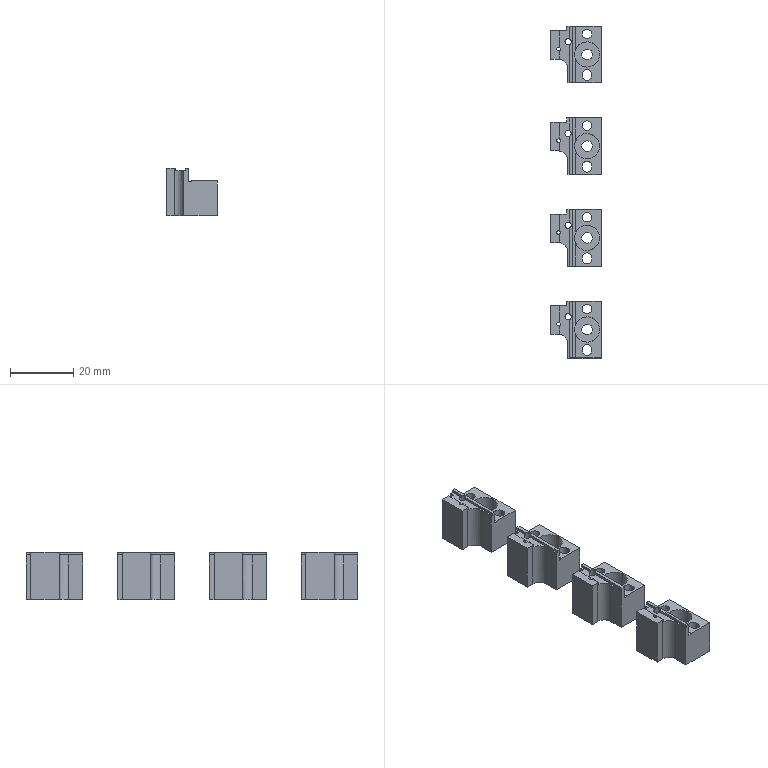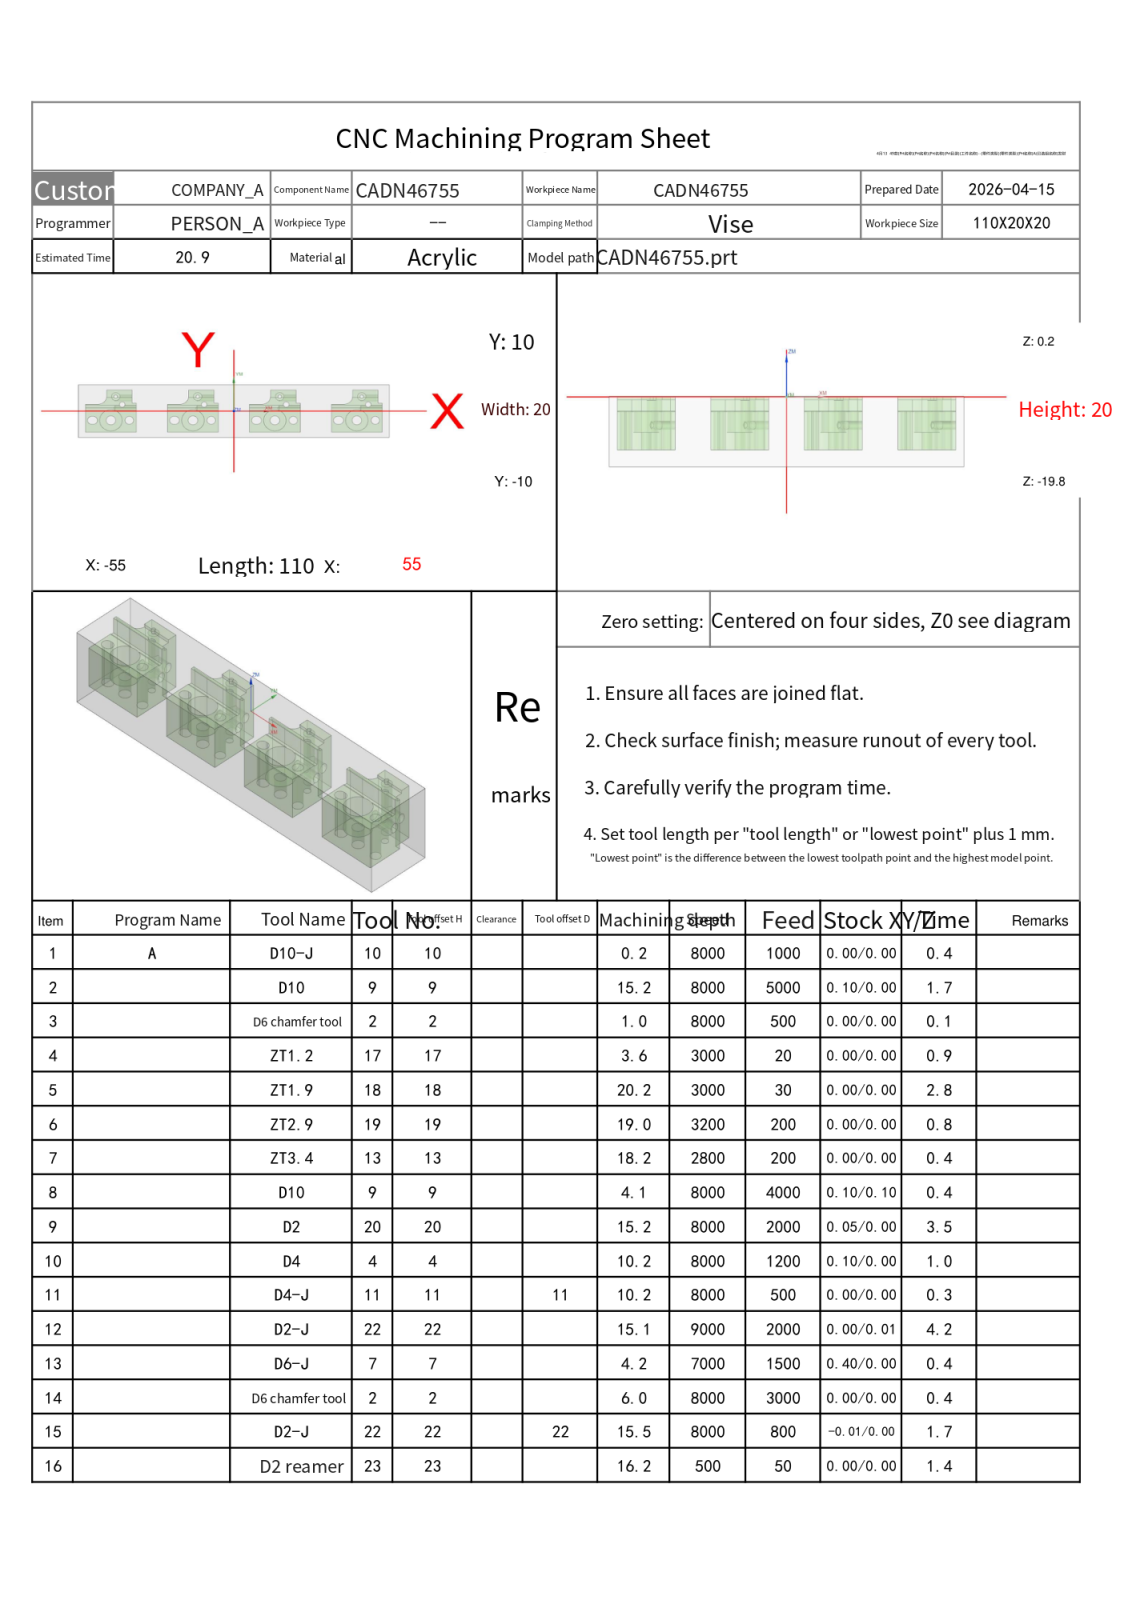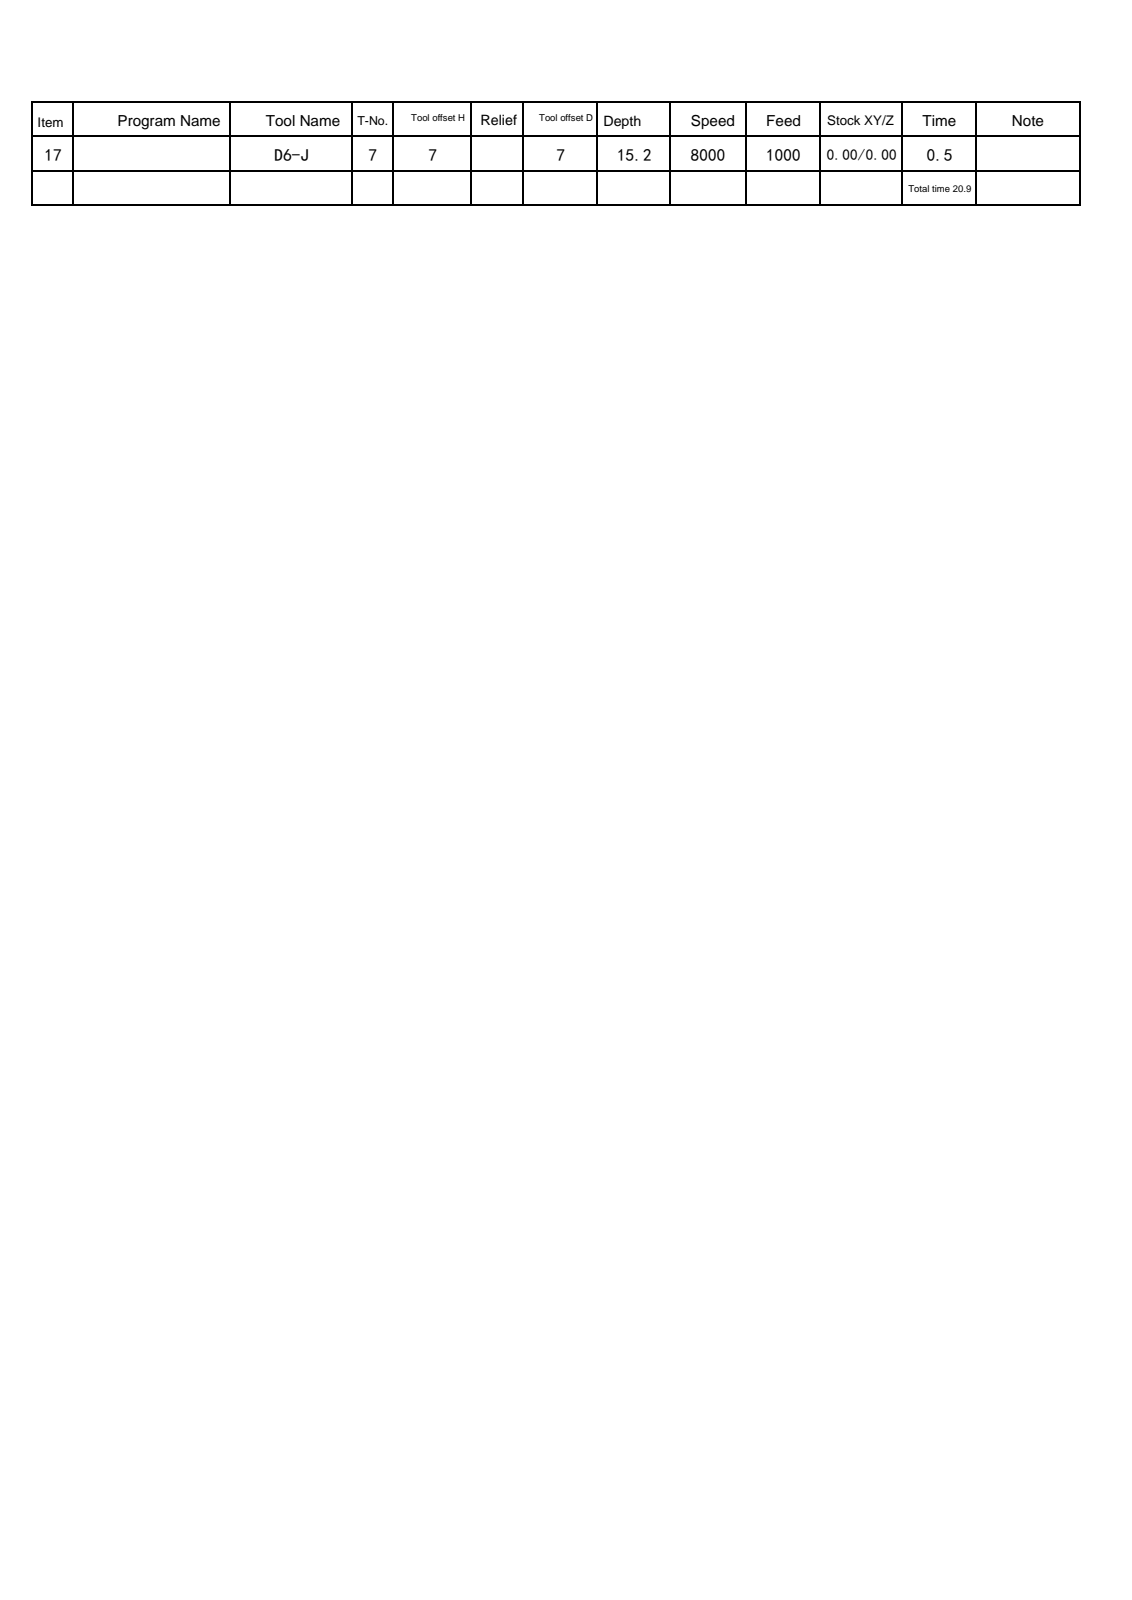NC program | NX | posted by the shop | part box 16 x 105 x 15 mm
Lines 1403 to 2192 of 25120:
N9 T20 M06
(D2  D=2. R=0. H=20 ce=0.10 di=0.00)
G00 G90 G54 X-50. Y-3.9 M03 S6000
G43 H20 Z20.
M08
Z-3.5
G01 X-49.75 Z-3.507 F600.
G03 X-49.35 Y-3.5 Z-3.525 I0.0 J.4
X-49.75 Y-3.1 Z-3.543 I-.4 J0.0
G01 X-50.25 Z-3.557
G03 X-50.65 Y-3.5 Z-3.574 I0.0 J-.4
X-50.559 Y-3.754 Z-3.582 I.4 J0.0
X-50.25 Y-3.9 Z-3.592 I.309 J.254
G01 X-49.75 Z-3.606
G03 X-49.35 Y-3.5 Z-3.624 I0.0 J.4
X-49.75 Y-3.1 Z-3.642 I-.4 J0.0
G01 X-50.25 Z-3.656
G03 X-50.65 Y-3.5 Z-3.673 I0.0 J-.4
X-50.559 Y-3.754 Z-3.681 I.4 J0.0
X-50.25 Y-3.9 Z-3.691 I.309 J.254
G01 X-49.75 Z-3.705
G03 X-49.35 Y-3.5 Z-3.723 I0.0 J.4
X-49.75 Y-3.1 Z-3.741 I-.4 J0.0
G01 X-50.25 Z-3.755
G03 X-50.65 Y-3.5 Z-3.773 I0.0 J-.4
X-50.559 Y-3.754 Z-3.78 I.4 J0.0
X-50.25 Y-3.9 Z-3.79 I.309 J.254
G01 X-49.75 Z-3.804
G03 X-49.35 Y-3.5 Z-3.822 I0.0 J.4
X-49.75 Y-3.1 Z-3.84 I-.4 J0.0
G01 X-50.25 Z-3.854
G03 X-50.65 Y-3.5 Z-3.872 I0.0 J-.4
X-50.559 Y-3.754 Z-3.88 I.4 J0.0
X-50.25 Y-3.9 Z-3.889 I.309 J.254
G01 X-49.75 Z-3.904
G03 X-49.35 Y-3.5 Z-3.921 I0.0 J.4
X-49.75 Y-3.1 Z-3.939 I-.4 J0.0
G01 X-50.25 Z-3.953
G03 X-50.65 Y-3.5 Z-3.971 I0.0 J-.4
X-50.559 Y-3.754 Z-3.979 I.4 J0.0
X-50.25 Y-3.9 Z-3.989 I.309 J.254
G01 X-49.75 Z-4.003
G03 X-49.35 Y-3.5 Z-4.02 I0.0 J.4
X-49.75 Y-3.1 Z-4.038 I-.4 J0.0
G01 X-50.25 Z-4.052
G03 X-50.65 Y-3.5 Z-4.07 I0.0 J-.4
X-50.559 Y-3.754 Z-4.078 I.4 J0.0
X-50.25 Y-3.9 Z-4.088 I.309 J.254
G01 X-49.75 Z-4.102
G03 X-49.35 Y-3.5 Z-4.12 I0.0 J.4
X-49.75 Y-3.1 Z-4.137 I-.4 J0.0
G01 X-50.25 Z-4.151
G03 X-50.65 Y-3.5 Z-4.169 I0.0 J-.4
X-50.559 Y-3.754 Z-4.177 I.4 J0.0
X-50.25 Y-3.9 Z-4.187 I.309 J.254
G01 X-49.75 Z-4.201
G03 X-49.35 Y-3.5 Z-4.219 I0.0 J.4
X-49.75 Y-3.1 Z-4.236 I-.4 J0.0
G01 X-50.25 Z-4.251
G03 X-50.65 Y-3.5 Z-4.268 I0.0 J-.4
X-50.559 Y-3.754 Z-4.276 I.4 J0.0
X-50.25 Y-3.9 Z-4.286 I.309 J.254
G01 X-49.75 Z-4.3
G03 X-49.35 Y-3.5 Z-4.318 I0.0 J.4
X-49.75 Y-3.1 Z-4.336 I-.4 J0.0
G01 X-50.25 Z-4.35
G03 X-50.65 Y-3.5 Z-4.367 I0.0 J-.4
X-50.559 Y-3.754 Z-4.375 I.4 J0.0
X-50.25 Y-3.9 Z-4.385 I.309 J.254
G01 X-49.75 Z-4.399
G03 X-49.35 Y-3.5 Z-4.417 I0.0 J.4
X-49.75 Y-3.1 Z-4.435 I-.4 J0.0
G01 X-50.25 Z-4.449
G03 X-50.65 Y-3.5 Z-4.467 I0.0 J-.4
X-50.559 Y-3.754 Z-4.474 I.4 J0.0
X-50.25 Y-3.9 Z-4.484 I.309 J.254
G01 X-49.75 Z-4.498
G03 X-49.35 Y-3.5 Z-4.516 I0.0 J.4
X-49.75 Y-3.1 Z-4.534 I-.4 J0.0
G01 X-50.25 Z-4.548
G03 X-50.65 Y-3.5 Z-4.566 I0.0 J-.4
X-50.559 Y-3.754 Z-4.574 I.4 J0.0
X-50.25 Y-3.9 Z-4.583 I.309 J.254
G01 X-49.75 Z-4.598
G03 X-49.35 Y-3.5 Z-4.615 I0.0 J.4
X-49.75 Y-3.1 Z-4.633 I-.4 J0.0
G01 X-50.25 Z-4.647
G03 X-50.65 Y-3.5 Z-4.665 I0.0 J-.4
X-50.559 Y-3.754 Z-4.673 I.4 J0.0
X-50.25 Y-3.9 Z-4.683 I.309 J.254
G01 X-49.75 Z-4.697
G03 X-49.35 Y-3.5 Z-4.714 I0.0 J.4
X-49.75 Y-3.1 Z-4.732 I-.4 J0.0
G01 X-50.25 Z-4.746
G03 X-50.65 Y-3.5 Z-4.764 I0.0 J-.4
X-50.559 Y-3.754 Z-4.772 I.4 J0.0
X-50.25 Y-3.9 Z-4.782 I.309 J.254
G01 X-49.75 Z-4.796
G03 X-49.35 Y-3.5 Z-4.814 I0.0 J.4
X-49.75 Y-3.1 Z-4.831 I-.4 J0.0
G01 X-50.25 Z-4.845
G03 X-50.65 Y-3.5 Z-4.863 I0.0 J-.4
X-50.559 Y-3.754 Z-4.871 I.4 J0.0
X-50.25 Y-3.9 Z-4.881 I.309 J.254
G01 X-49.75 Z-4.895
G03 X-49.35 Y-3.5 Z-4.913 I0.0 J.4
X-49.75 Y-3.1 Z-4.93 I-.4 J0.0
G01 X-50.25 Z-4.945
G03 X-50.65 Y-3.5 Z-4.962 I0.0 J-.4
X-50.559 Y-3.754 Z-4.97 I.4 J0.0
X-50.25 Y-3.9 Z-4.98 I.309 J.254
G01 X-49.75 Z-4.994
G03 X-49.35 Y-3.5 Z-5.012 I0.0 J.4
X-49.75 Y-3.1 Z-5.03 I-.4 J0.0
G01 X-50.25 Z-5.044
G03 X-50.65 Y-3.5 Z-5.061 I0.0 J-.4
X-50.559 Y-3.754 Z-5.069 I.4 J0.0
X-50.25 Y-3.9 Z-5.079 I.309 J.254
G01 X-49.75 Z-5.093
G03 X-49.35 Y-3.5 Z-5.111 I0.0 J.4
X-49.75 Y-3.1 Z-5.129 I-.4 J0.0
G01 X-50.25 Z-5.143
G03 X-50.65 Y-3.5 Z-5.161 I0.0 J-.4
X-50.559 Y-3.754 Z-5.168 I.4 J0.0
X-50.25 Y-3.9 Z-5.178 I.309 J.254
G01 X-49.75 Z-5.192
G03 X-49.35 Y-3.5 Z-5.21 I0.0 J.4
X-49.75 Y-3.1 Z-5.228 I-.4 J0.0
G01 X-50.25 Z-5.242
G03 X-50.65 Y-3.5 Z-5.26 I0.0 J-.4
X-50.559 Y-3.754 Z-5.267 I.4 J0.0
X-50.25 Y-3.9 Z-5.277 I.309 J.254
G01 X-49.75 Z-5.292
G03 X-49.35 Y-3.5 Z-5.309 I0.0 J.4
X-49.75 Y-3.1 Z-5.327 I-.4 J0.0
G01 X-50.25 Z-5.341
G03 X-50.65 Y-3.5 Z-5.359 I0.0 J-.4
X-50.559 Y-3.754 Z-5.367 I.4 J0.0
X-50.25 Y-3.9 Z-5.377 I.309 J.254
G01 X-49.75 Z-5.391
G03 X-49.35 Y-3.5 Z-5.408 I0.0 J.4
X-49.75 Y-3.1 Z-5.426 I-.4 J0.0
G01 X-50.25 Z-5.44
G03 X-50.65 Y-3.5 Z-5.458 I0.0 J-.4
X-50.559 Y-3.754 Z-5.466 I.4 J0.0
X-50.25 Y-3.9 Z-5.476 I.309 J.254
G01 X-49.75 Z-5.49
G03 X-49.35 Y-3.5 Z-5.508 I0.0 J.4
X-49.75 Y-3.1 Z-5.525 I-.4 J0.0
G01 X-50.25 Z-5.539
G03 X-50.65 Y-3.5 Z-5.557 I0.0 J-.4
X-50.559 Y-3.754 Z-5.565 I.4 J0.0
X-50.25 Y-3.9 Z-5.575 I.309 J.254
G01 X-49.75 Z-5.589
G03 X-49.35 Y-3.5 Z-5.607 I0.0 J.4
X-49.75 Y-3.1 Z-5.624 I-.4 J0.0
G01 X-50.25 Z-5.639
G03 X-50.65 Y-3.5 Z-5.656 I0.0 J-.4
X-50.559 Y-3.754 Z-5.664 I.4 J0.0
X-50.25 Y-3.9 Z-5.674 I.309 J.254
G01 X-49.75 Z-5.688
G03 X-49.35 Y-3.5 Z-5.706 I0.0 J.4
X-49.75 Y-3.1 Z-5.724 I-.4 J0.0
G01 X-50.25 Z-5.738
G03 X-50.65 Y-3.5 Z-5.755 I0.0 J-.4
X-50.559 Y-3.754 Z-5.763 I.4 J0.0
X-50.25 Y-3.9 Z-5.773 I.309 J.254
G01 X-49.75 Z-5.787
G03 X-49.35 Y-3.5 Z-5.805 I0.0 J.4
X-49.75 Y-3.1 Z-5.823 I-.4 J0.0
G01 X-50.25 Z-5.837
G03 X-50.65 Y-3.5 Z-5.855 I0.0 J-.4
X-50.559 Y-3.754 Z-5.862 I.4 J0.0
X-50.25 Y-3.9 Z-5.872 I.309 J.254
G01 X-49.75 Z-5.886
G03 X-49.35 Y-3.5 Z-5.904 I0.0 J.4
X-49.75 Y-3.1 Z-5.922 I-.4 J0.0
G01 X-50.25 Z-5.936
G03 X-50.65 Y-3.5 Z-5.954 I0.0 J-.4
X-50.559 Y-3.754 Z-5.961 I.4 J0.0
X-50.25 Y-3.9 Z-5.971 I.309 J.254
G01 X-49.75 Z-5.986
G03 X-49.35 Y-3.5 Z-6.003 I0.0 J.4
X-49.75 Y-3.1 Z-6.021 I-.4 J0.0
G01 X-50.25 Z-6.035
G03 X-50.65 Y-3.5 Z-6.053 I0.0 J-.4
X-50.559 Y-3.754 Z-6.061 I.4 J0.0
X-50.25 Y-3.9 Z-6.071 I.309 J.254
G01 X-49.75 Z-6.085
G03 X-49.35 Y-3.5 Z-6.102 I0.0 J.4
X-49.75 Y-3.1 Z-6.12 I-.4 J0.0
G01 X-50.25 Z-6.134
G03 X-50.65 Y-3.5 Z-6.152 I0.0 J-.4
X-50.559 Y-3.754 Z-6.16 I.4 J0.0
X-50.25 Y-3.9 Z-6.17 I.309 J.254
G01 X-49.75 Z-6.184
G03 X-49.35 Y-3.5 Z-6.202 I0.0 J.4
X-49.75 Y-3.1 Z-6.219 I-.4 J0.0
G01 X-50.25 Z-6.233
G03 X-50.65 Y-3.5 Z-6.251 I0.0 J-.4
X-50.559 Y-3.754 Z-6.259 I.4 J0.0
X-50.25 Y-3.9 Z-6.269 I.309 J.254
G01 X-49.75 Z-6.283
G03 X-49.35 Y-3.5 Z-6.301 I0.0 J.4
X-49.75 Y-3.1 Z-6.318 I-.4 J0.0
G01 X-50.25 Z-6.332
G03 X-50.65 Y-3.5 Z-6.35 I0.0 J-.4
X-50.559 Y-3.754 Z-6.358 I.4 J0.0
X-50.25 Y-3.9 Z-6.368 I.309 J.254
G01 X-49.75 Z-6.382
G03 X-49.35 Y-3.5 Z-6.4 I0.0 J.4
X-49.75 Y-3.1 Z-6.418 I-.4 J0.0
G01 X-50.25 Z-6.432
G03 X-50.65 Y-3.5 Z-6.449 I0.0 J-.4
X-50.559 Y-3.754 Z-6.457 I.4 J0.0
X-50.25 Y-3.9 Z-6.467 I.309 J.254
G01 X-49.75 Z-6.481
G03 X-49.35 Y-3.5 Z-6.499 I0.0 J.4
X-49.75 Y-3.1 Z-6.517 I-.4 J0.0
G01 X-50.25 Z-6.531
G03 X-50.65 Y-3.5 Z-6.548 I0.0 J-.4
X-50.559 Y-3.754 Z-6.556 I.4 J0.0
X-50.25 Y-3.9 Z-6.566 I.309 J.254
G01 X-49.75 Z-6.58
G03 X-49.35 Y-3.5 Z-6.598 I0.0 J.4
X-49.75 Y-3.1 Z-6.616 I-.4 J0.0
G01 X-50.25 Z-6.63
G03 X-50.65 Y-3.5 Z-6.648 I0.0 J-.4
X-50.559 Y-3.754 Z-6.655 I.4 J0.0
X-50.25 Y-3.9 Z-6.665 I.309 J.254
G01 X-49.75 Z-6.679
G03 X-49.35 Y-3.5 Z-6.697 I0.0 J.4
X-49.75 Y-3.1 Z-6.715 I-.4 J0.0
G01 X-50.25 Z-6.729
G03 X-50.65 Y-3.5 Z-6.747 I0.0 J-.4
X-50.559 Y-3.754 Z-6.755 I.4 J0.0
X-50.25 Y-3.9 Z-6.764 I.309 J.254
G01 X-49.75 Z-6.779
G03 X-49.35 Y-3.5 Z-6.796 I0.0 J.4
X-49.75 Y-3.1 Z-6.814 I-.4 J0.0
G01 X-50.25 Z-6.828
G03 X-50.65 Y-3.5 Z-6.846 I0.0 J-.4
X-50.559 Y-3.754 Z-6.854 I.4 J0.0
X-50.25 Y-3.9 Z-6.864 I.309 J.254
G01 X-49.75 Z-6.878
G03 X-49.35 Y-3.5 Z-6.895 I0.0 J.4
X-49.75 Y-3.1 Z-6.913 I-.4 J0.0
G01 X-50.25 Z-6.927
G03 X-50.65 Y-3.5 Z-6.945 I0.0 J-.4
X-50.559 Y-3.754 Z-6.953 I.4 J0.0
X-50.25 Y-3.9 Z-6.963 I.309 J.254
G01 X-49.75 Z-6.977
G03 X-49.35 Y-3.5 Z-6.995 I0.0 J.4
X-49.75 Y-3.1 Z-7.012 I-.4 J0.0
G01 X-50.25 Z-7.026
G03 X-50.65 Y-3.5 Z-7.044 I0.0 J-.4
X-50.559 Y-3.754 Z-7.052 I.4 J0.0
X-50.25 Y-3.9 Z-7.062 I.309 J.254
G01 X-49.75 Z-7.076
G03 X-49.35 Y-3.5 Z-7.094 I0.0 J.4
X-49.75 Y-3.1 Z-7.111 I-.4 J0.0
G01 X-50.25 Z-7.126
G03 X-50.65 Y-3.5 Z-7.143 I0.0 J-.4
X-50.559 Y-3.754 Z-7.151 I.4 J0.0
X-50.25 Y-3.9 Z-7.161 I.309 J.254
G01 X-49.75 Z-7.175
G03 X-49.35 Y-3.5 Z-7.193 I0.0 J.4
X-49.75 Y-3.1 Z-7.211 I-.4 J0.0
G01 X-50.25 Z-7.225
G03 X-50.65 Y-3.5 Z-7.242 I0.0 J-.4
X-50.559 Y-3.754 Z-7.25 I.4 J0.0
X-50.25 Y-3.9 Z-7.26 I.309 J.254
G01 X-49.75 Z-7.274
G03 X-49.35 Y-3.5 Z-7.292 I0.0 J.4
X-49.75 Y-3.1 Z-7.31 I-.4 J0.0
G01 X-50.25 Z-7.324
G03 X-50.65 Y-3.5 Z-7.342 I0.0 J-.4
X-50.559 Y-3.754 Z-7.349 I.4 J0.0
X-50.25 Y-3.9 Z-7.359 I.309 J.254
G01 X-49.75 Z-7.373
G03 X-49.35 Y-3.5 Z-7.391 I0.0 J.4
X-49.75 Y-3.1 Z-7.409 I-.4 J0.0
G01 X-50.25 Z-7.423
G03 X-50.65 Y-3.5 Z-7.441 I0.0 J-.4
X-50.559 Y-3.754 Z-7.449 I.4 J0.0
X-50.25 Y-3.9 Z-7.458 I.309 J.254
G01 X-49.75 Z-7.473
G03 X-49.35 Y-3.5 Z-7.49 I0.0 J.4
X-49.75 Y-3.1 Z-7.508 I-.4 J0.0
G01 X-50.25 Z-7.522
G03 X-50.65 Y-3.5 Z-7.54 I0.0 J-.4
X-50.559 Y-3.754 Z-7.548 I.4 J0.0
X-50.25 Y-3.9 Z-7.558 I.309 J.254
G01 X-49.75 Z-7.572
G03 X-49.35 Y-3.5 Z-7.589 I0.0 J.4
X-49.75 Y-3.1 Z-7.607 I-.4 J0.0
G01 X-50.25 Z-7.621
G03 X-50.65 Y-3.5 Z-7.639 I0.0 J-.4
X-50.559 Y-3.754 Z-7.647 I.4 J0.0
X-50.25 Y-3.9 Z-7.657 I.309 J.254
G01 X-49.75 Z-7.671
G03 X-49.35 Y-3.5 Z-7.689 I0.0 J.4
X-49.75 Y-3.1 Z-7.706 I-.4 J0.0
G01 X-50.25 Z-7.72
G03 X-50.65 Y-3.5 Z-7.738 I0.0 J-.4
X-50.559 Y-3.754 Z-7.746 I.4 J0.0
X-50.25 Y-3.9 Z-7.756 I.309 J.254
G01 X-49.75 Z-7.77
G03 X-49.35 Y-3.5 Z-7.788 I0.0 J.4
X-49.75 Y-3.1 Z-7.805 I-.4 J0.0
G01 X-50.25 Z-7.82
G03 X-50.65 Y-3.5 Z-7.837 I0.0 J-.4
X-50.559 Y-3.754 Z-7.845 I.4 J0.0
X-50.25 Y-3.9 Z-7.855 I.309 J.254
G01 X-49.75 Z-7.869
G03 X-49.35 Y-3.5 Z-7.887 I0.0 J.4
X-49.75 Y-3.1 Z-7.905 I-.4 J0.0
G01 X-50.25 Z-7.919
G03 X-50.65 Y-3.5 Z-7.936 I0.0 J-.4
X-50.559 Y-3.754 Z-7.944 I.4 J0.0
X-50.25 Y-3.9 Z-7.954 I.309 J.254
G01 X-49.75 Z-7.968
G03 X-49.35 Y-3.5 Z-7.986 I0.0 J.4
X-49.75 Y-3.1 Z-8.004 I-.4 J0.0
G01 X-50.25 Z-8.018
G03 X-50.65 Y-3.5 Z-8.036 I0.0 J-.4
X-50.559 Y-3.754 Z-8.043 I.4 J0.0
X-50.25 Y-3.9 Z-8.053 I.309 J.254
G01 X-49.75 Z-8.067
G03 X-49.35 Y-3.5 Z-8.085 I0.0 J.4
X-49.75 Y-3.1 Z-8.103 I-.4 J0.0
G01 X-50.25 Z-8.117
G03 X-50.65 Y-3.5 Z-8.135 I0.0 J-.4
X-50.559 Y-3.754 Z-8.142 I.4 J0.0
X-50.25 Y-3.9 Z-8.152 I.309 J.254
G01 X-49.75 Z-8.167
G03 X-49.35 Y-3.5 Z-8.184 I0.0 J.4
X-49.75 Y-3.1 Z-8.202 I-.4 J0.0
G01 X-50.25 Z-8.216
G03 X-50.65 Y-3.5 Z-8.234 I0.0 J-.4
X-50.559 Y-3.754 Z-8.242 I.4 J0.0
X-50.25 Y-3.9 Z-8.252 I.309 J.254
G01 X-49.75 Z-8.266
G03 X-49.35 Y-3.5 Z-8.283 I0.0 J.4
X-49.75 Y-3.1 Z-8.301 I-.4 J0.0
G01 X-50.25 Z-8.315
G03 X-50.65 Y-3.5 Z-8.333 I0.0 J-.4
X-50.559 Y-3.754 Z-8.341 I.4 J0.0
X-50.25 Y-3.9 Z-8.351 I.309 J.254
G01 X-49.75 Z-8.365
G03 X-49.35 Y-3.5 Z-8.383 I0.0 J.4
X-49.75 Y-3.1 Z-8.4 I-.4 J0.0
G01 X-50.25 Z-8.414
G03 X-50.65 Y-3.5 Z-8.432 I0.0 J-.4
X-50.559 Y-3.754 Z-8.44 I.4 J0.0
X-50.25 Y-3.9 Z-8.45 I.309 J.254
G01 X-49.75 Z-8.464
G03 X-49.35 Y-3.5 Z-8.482 I0.0 J.4
X-49.75 Y-3.1 Z-8.499 I-.4 J0.0
G01 X-50.25 Z-8.514
G03 X-50.65 Y-3.5 Z-8.531 I0.0 J-.4
X-50.559 Y-3.754 Z-8.539 I.4 J0.0
X-50.25 Y-3.9 Z-8.549 I.309 J.254
G01 X-49.75 Z-8.563
G03 X-49.35 Y-3.5 Z-8.581 I0.0 J.4
X-49.75 Y-3.1 Z-8.599 I-.4 J0.0
G01 X-50.25 Z-8.613
G03 X-50.65 Y-3.5 Z-8.63 I0.0 J-.4
X-50.559 Y-3.754 Z-8.638 I.4 J0.0
X-50.25 Y-3.9 Z-8.648 I.309 J.254
G01 X-49.75 Z-8.662
G03 X-49.35 Y-3.5 Z-8.68 I0.0 J.4
X-49.75 Y-3.1 Z-8.698 I-.4 J0.0
G01 X-50.25 Z-8.712
G03 X-50.65 Y-3.5 Z-8.73 I0.0 J-.4
X-50.559 Y-3.754 Z-8.737 I.4 J0.0
X-50.25 Y-3.9 Z-8.747 I.309 J.254
G01 X-49.75 Z-8.761
G03 X-49.35 Y-3.5 Z-8.779 I0.0 J.4
X-49.75 Y-3.1 Z-8.797 I-.4 J0.0
G01 X-50.25 Z-8.811
G03 X-50.65 Y-3.5 Z-8.829 I0.0 J-.4
X-50.559 Y-3.754 Z-8.836 I.4 J0.0
X-50.25 Y-3.9 Z-8.846 I.309 J.254
G01 X-49.75 Z-8.861
G03 X-49.35 Y-3.5 Z-8.878 I0.0 J.4
X-49.75 Y-3.1 Z-8.896 I-.4 J0.0
G01 X-50.25 Z-8.91
G03 X-50.65 Y-3.5 Z-8.928 I0.0 J-.4
X-50.559 Y-3.754 Z-8.936 I.4 J0.0
X-50.25 Y-3.9 Z-8.946 I.309 J.254
G01 X-49.75 Z-8.96
G03 X-49.35 Y-3.5 Z-8.977 I0.0 J.4
X-49.75 Y-3.1 Z-8.995 I-.4 J0.0
G01 X-50.25 Z-9.009
G03 X-50.65 Y-3.5 Z-9.027 I0.0 J-.4
X-50.559 Y-3.754 Z-9.035 I.4 J0.0
X-50.25 Y-3.9 Z-9.045 I.309 J.254
G01 X-49.75 Z-9.059
G03 X-49.35 Y-3.5 Z-9.077 I0.0 J.4
X-49.75 Y-3.1 Z-9.094 I-.4 J0.0
G01 X-50.25 Z-9.108
G03 X-50.65 Y-3.5 Z-9.126 I0.0 J-.4
X-50.559 Y-3.754 Z-9.134 I.4 J0.0
X-50.25 Y-3.9 Z-9.144 I.309 J.254
G01 X-49.75 Z-9.158
G03 X-49.35 Y-3.5 Z-9.176 I0.0 J.4
X-49.75 Y-3.1 Z-9.193 I-.4 J0.0
G01 X-50.25 Z-9.207
G03 X-50.65 Y-3.5 Z-9.225 I0.0 J-.4
X-50.559 Y-3.754 Z-9.233 I.4 J0.0
X-50.25 Y-3.9 Z-9.243 I.309 J.254
G01 X-49.75 Z-9.257
G03 X-49.35 Y-3.5 Z-9.275 I0.0 J.4
X-49.75 Y-3.1 Z-9.293 I-.4 J0.0
G01 X-50.25 Z-9.307
G03 X-50.65 Y-3.5 Z-9.324 I0.0 J-.4
X-50.559 Y-3.754 Z-9.332 I.4 J0.0
X-50.25 Y-3.9 Z-9.342 I.309 J.254
G01 X-49.75 Z-9.356
G03 X-49.35 Y-3.5 Z-9.374 I0.0 J.4
X-49.75 Y-3.1 Z-9.392 I-.4 J0.0
G01 X-50.25 Z-9.406
G03 X-50.65 Y-3.5 Z-9.423 I0.0 J-.4
X-50.559 Y-3.754 Z-9.431 I.4 J0.0
X-50.25 Y-3.9 Z-9.441 I.309 J.254
G01 X-49.75 Z-9.455
G03 X-49.35 Y-3.5 Z-9.473 I0.0 J.4
X-49.75 Y-3.1 Z-9.491 I-.4 J0.0
G01 X-50.25 Z-9.505
G03 X-50.65 Y-3.5 Z-9.523 I0.0 J-.4
X-50.559 Y-3.754 Z-9.53 I.4 J0.0
X-50.25 Y-3.9 Z-9.54 I.309 J.254
G01 X-49.75 Z-9.554
G03 X-49.35 Y-3.5 Z-9.572 I0.0 J.4
X-49.75 Y-3.1 Z-9.59 I-.4 J0.0
G01 X-50.25 Z-9.604
G03 X-50.65 Y-3.5 Z-9.622 I0.0 J-.4
X-50.559 Y-3.754 Z-9.63 I.4 J0.0
X-50.25 Y-3.9 Z-9.639 I.309 J.254
G01 X-49.75 Z-9.654
G03 X-49.35 Y-3.5 Z-9.671 I0.0 J.4
X-49.75 Y-3.1 Z-9.689 I-.4 J0.0
G01 X-50.25 Z-9.703
G03 X-50.65 Y-3.5 Z-9.721 I0.0 J-.4
X-50.559 Y-3.754 Z-9.729 I.4 J0.0
X-50.25 Y-3.9 Z-9.739 I.309 J.254
G01 X-49.75 Z-9.753
G03 X-49.35 Y-3.5 Z-9.77 I0.0 J.4
X-49.75 Y-3.1 Z-9.788 I-.4 J0.0
G01 X-50.25 Z-9.802
G03 X-50.65 Y-3.5 Z-9.82 I0.0 J-.4
X-50.559 Y-3.754 Z-9.828 I.4 J0.0
X-50.25 Y-3.9 Z-9.838 I.309 J.254
G01 X-49.75 Z-9.852
G03 X-49.35 Y-3.5 Z-9.87 I0.0 J.4
X-49.75 Y-3.1 Z-9.887 I-.4 J0.0
G01 X-50.25 Z-9.901
G03 X-50.65 Y-3.5 Z-9.919 I0.0 J-.4
X-50.559 Y-3.754 Z-9.927 I.4 J0.0
X-50.25 Y-3.9 Z-9.937 I.309 J.254
G01 X-49.75 Z-9.951
G03 X-49.35 Y-3.5 Z-9.969 I0.0 J.4
X-49.75 Y-3.1 Z-9.986 I-.4 J0.0
G01 X-50.25 Z-10.001
G03 X-50.65 Y-3.5 Z-10.018 I0.0 J-.4
X-50.559 Y-3.754 Z-10.026 I.4 J0.0
X-50.25 Y-3.9 Z-10.036 I.309 J.254
G01 X-49.75 Z-10.05
G03 X-49.35 Y-3.5 Z-10.068 I0.0 J.4
X-49.75 Y-3.1 Z-10.086 I-.4 J0.0
G01 X-50.25 Z-10.1
G03 X-50.65 Y-3.5 Z-10.117 I0.0 J-.4
X-50.559 Y-3.754 Z-10.125 I.4 J0.0
X-50.25 Y-3.9 Z-10.135 I.309 J.254
G01 X-49.75 Z-10.149
G03 X-49.35 Y-3.5 Z-10.167 I0.0 J.4
X-49.75 Y-3.1 Z-10.185 I-.4 J0.0
G01 X-50.25 Z-10.199
G03 X-50.65 Y-3.5 Z-10.217 I0.0 J-.4
X-50.559 Y-3.754 Z-10.224 I.4 J0.0
X-50.25 Y-3.9 Z-10.234 I.309 J.254
G01 X-49.75 Z-10.248
G03 X-49.35 Y-3.5 Z-10.266 I0.0 J.4
X-49.75 Y-3.1 Z-10.284 I-.4 J0.0
G01 X-50.25 Z-10.298
G03 X-50.65 Y-3.5 Z-10.316 I0.0 J-.4
X-50.559 Y-3.754 Z-10.324 I.4 J0.0
X-50.25 Y-3.9 Z-10.333 I.309 J.254
G01 X-49.75 Z-10.348
G03 X-49.35 Y-3.5 Z-10.365 I0.0 J.4
X-49.75 Y-3.1 Z-10.383 I-.4 J0.0
G01 X-50.25 Z-10.397
G03 X-50.65 Y-3.5 Z-10.415 I0.0 J-.4
X-50.559 Y-3.754 Z-10.423 I.4 J0.0
X-50.25 Y-3.9 Z-10.433 I.309 J.254
G01 X-49.75 Z-10.447
G03 X-49.35 Y-3.5 Z-10.464 I0.0 J.4
X-49.75 Y-3.1 Z-10.482 I-.4 J0.0
G01 X-50.25 Z-10.496
G03 X-50.65 Y-3.5 Z-10.514 I0.0 J-.4
X-50.559 Y-3.754 Z-10.522 I.4 J0.0
X-50.25 Y-3.9 Z-10.532 I.309 J.254
G01 X-49.75 Z-10.546
G03 X-49.35 Y-3.5 Z-10.564 I0.0 J.4
X-49.75 Y-3.1 Z-10.581 I-.4 J0.0
G01 X-50.25 Z-10.595
G03 X-50.65 Y-3.5 Z-10.613 I0.0 J-.4
X-50.559 Y-3.754 Z-10.621 I.4 J0.0
X-50.25 Y-3.9 Z-10.631 I.309 J.254
G01 X-49.75 Z-10.645
G03 X-49.35 Y-3.5 Z-10.663 I0.0 J.4
X-49.75 Y-3.1 Z-10.68 I-.4 J0.0
G01 X-50.25 Z-10.695
G03 X-50.65 Y-3.5 Z-10.712 I0.0 J-.4
X-50.559 Y-3.754 Z-10.72 I.4 J0.0
X-50.25 Y-3.9 Z-10.73 I.309 J.254
G01 X-49.75 Z-10.744
G03 X-49.35 Y-3.5 Z-10.762 I0.0 J.4
X-49.75 Y-3.1 Z-10.78 I-.4 J0.0
G01 X-50.25 Z-10.794
G03 X-50.65 Y-3.5 Z-10.811 I0.0 J-.4
X-50.559 Y-3.754 Z-10.819 I.4 J0.0
X-50.25 Y-3.9 Z-10.829 I.309 J.254
G01 X-49.75 Z-10.843
G03 X-49.35 Y-3.5 Z-10.861 I0.0 J.4
X-49.75 Y-3.1 Z-10.879 I-.4 J0.0
G01 X-50.25 Z-10.893
G03 X-50.65 Y-3.5 Z-10.911 I0.0 J-.4
X-50.559 Y-3.754 Z-10.918 I.4 J0.0
X-50.25 Y-3.9 Z-10.928 I.309 J.254
G01 X-49.75 Z-10.942
G03 X-49.35 Y-3.5 Z-10.96 I0.0 J.4
X-49.75 Y-3.1 Z-10.978 I-.4 J0.0
G01 X-50.25 Z-10.992
G03 X-50.65 Y-3.5 Z-11.01 I0.0 J-.4
X-50.559 Y-3.754 Z-11.017 I.4 J0.0
X-50.25 Y-3.9 Z-11.027 I.309 J.254
G01 X-49.75 Z-11.042
G03 X-49.35 Y-3.5 Z-11.059 I0.0 J.4
X-49.75 Y-3.1 Z-11.077 I-.4 J0.0
G01 X-50.25 Z-11.091
G03 X-50.65 Y-3.5 Z-11.109 I0.0 J-.4
X-50.559 Y-3.754 Z-11.117 I.4 J0.0
X-50.25 Y-3.9 Z-11.127 I.309 J.254
G01 X-49.75 Z-11.141
G03 X-49.35 Y-3.5 Z-11.158 I0.0 J.4
X-49.75 Y-3.1 Z-11.176 I-.4 J0.0
G01 X-50.25 Z-11.19
G03 X-50.65 Y-3.5 Z-11.208 I0.0 J-.4
X-50.559 Y-3.754 Z-11.216 I.4 J0.0
X-50.25 Y-3.9 Z-11.226 I.309 J.254
G01 X-49.75 Z-11.24
G03 X-49.35 Y-3.5 Z-11.258 I0.0 J.4
X-49.75 Y-3.1 Z-11.275 I-.4 J0.0
G01 X-50.25 Z-11.289
G03 X-50.65 Y-3.5 Z-11.307 I0.0 J-.4
X-50.559 Y-3.754 Z-11.315 I.4 J0.0
X-50.25 Y-3.9 Z-11.325 I.309 J.254
G01 X-49.75 Z-11.339
G03 X-49.35 Y-3.5 Z-11.357 I0.0 J.4
X-49.75 Y-3.1 Z-11.374 I-.4 J0.0
G01 X-50.25 Z-11.389
G03 X-50.65 Y-3.5 Z-11.406 I0.0 J-.4
X-50.559 Y-3.754 Z-11.414 I.4 J0.0
X-50.25 Y-3.9 Z-11.424 I.309 J.254
G01 X-49.75 Z-11.438
G03 X-49.35 Y-3.5 Z-11.456 I0.0 J.4
X-49.75 Y-3.1 Z-11.474 I-.4 J0.0
G01 X-50.25 Z-11.488
G03 X-50.65 Y-3.5 Z-11.505 I0.0 J-.4
X-50.559 Y-3.754 Z-11.513 I.4 J0.0
X-50.25 Y-3.9 Z-11.523 I.309 J.254
G01 X-49.75 Z-11.537
G03 X-49.35 Y-3.5 Z-11.555 I0.0 J.4
X-49.75 Y-3.1 Z-11.573 I-.4 J0.0
G01 X-50.25 Z-11.587
G03 X-50.65 Y-3.5 Z-11.605 I0.0 J-.4
X-50.559 Y-3.754 Z-11.612 I.4 J0.0
X-50.25 Y-3.9 Z-11.622 I.309 J.254
G01 X-49.75 Z-11.636
G03 X-49.35 Y-3.5 Z-11.654 I0.0 J.4
X-49.75 Y-3.1 Z-11.672 I-.4 J0.0
G01 X-50.25 Z-11.686
G03 X-50.65 Y-3.5 Z-11.704 I0.0 J-.4
X-50.559 Y-3.754 Z-11.711 I.4 J0.0
X-50.25 Y-3.9 Z-11.721 I.309 J.254
G01 X-49.75 Z-11.736
G03 X-49.35 Y-3.5 Z-11.753 I0.0 J.4
X-49.75 Y-3.1 Z-11.771 I-.4 J0.0
G01 X-50.25 Z-11.785
G03 X-50.65 Y-3.5 Z-11.803 I0.0 J-.4
X-50.559 Y-3.754 Z-11.811 I.4 J0.0
X-50.25 Y-3.9 Z-11.821 I.309 J.254
G01 X-49.75 Z-11.835
G03 X-49.35 Y-3.5 Z-11.852 I0.0 J.4
X-49.75 Y-3.1 Z-11.87 I-.4 J0.0
G01 X-50.25 Z-11.884
G03 X-50.65 Y-3.5 Z-11.902 I0.0 J-.4
X-50.559 Y-3.754 Z-11.91 I.4 J0.0
X-50.25 Y-3.9 Z-11.92 I.309 J.254
G01 X-49.75 Z-11.934
G03 X-49.35 Y-3.5 Z-11.952 I0.0 J.4
X-49.75 Y-3.1 Z-11.969 I-.4 J0.0
G01 X-50.25 Z-11.983
G03 X-50.65 Y-3.5 Z-12.001 I0.0 J-.4
X-50.559 Y-3.754 Z-12.009 I.4 J0.0
X-50.25 Y-3.9 Z-12.019 I.309 J.254
G01 X-49.75 Z-12.033
G03 X-49.35 Y-3.5 Z-12.051 I0.0 J.4
X-49.75 Y-3.1 Z-12.068 I-.4 J0.0
G01 X-50.25 Z-12.082
G03 X-50.65 Y-3.5 Z-12.1 I0.0 J-.4
X-50.559 Y-3.754 Z-12.108 I.4 J0.0
X-50.25 Y-3.9 Z-12.118 I.309 J.254
G01 X-49.75 Z-12.132
G03 X-49.35 Y-3.5 Z-12.15 I0.0 J.4
X-49.75 Y-3.1 Z-12.168 I-.4 J0.0
G01 X-50.25 Z-12.182
G03 X-50.65 Y-3.5 Z-12.199 I0.0 J-.4
X-50.559 Y-3.754 Z-12.207 I.4 J0.0
X-50.25 Y-3.9 Z-12.217 I.309 J.254
G01 X-49.75 Z-12.231
G03 X-49.35 Y-3.5 Z-12.249 I0.0 J.4
X-49.75 Y-3.1 Z-12.267 I-.4 J0.0
G01 X-50.25 Z-12.281
G03 X-50.65 Y-3.5 Z-12.298 I0.0 J-.4
X-50.559 Y-3.754 Z-12.306 I.4 J0.0
X-50.25 Y-3.9 Z-12.316 I.309 J.254
G01 X-49.75 Z-12.33
G03 X-49.35 Y-3.5 Z-12.348 I0.0 J.4
X-49.75 Y-3.1 Z-12.366 I-.4 J0.0
G01 X-50.25 Z-12.38
G03 X-50.65 Y-3.5 Z-12.398 I0.0 J-.4
X-50.559 Y-3.754 Z-12.405 I.4 J0.0
X-50.25 Y-3.9 Z-12.415 I.309 J.254
G01 X-49.75 Z-12.429
G03 X-49.35 Y-3.5 Z-12.447 I0.0 J.4
X-49.75 Y-3.1 Z-12.465 I-.4 J0.0
G01 X-50.25 Z-12.479
G03 X-50.65 Y-3.5 Z-12.497 I0.0 J-.4
X-50.559 Y-3.754 Z-12.505 I.4 J0.0
X-50.25 Y-3.9 Z-12.514 I.309 J.254
G01 X-49.75 Z-12.529
G03 X-49.35 Y-3.5 Z-12.546 I0.0 J.4
X-49.75 Y-3.1 Z-12.564 I-.4 J0.0
G01 X-50.25 Z-12.578
G03 X-50.65 Y-3.5 Z-12.596 I0.0 J-.4
X-50.559 Y-3.754 Z-12.604 I.4 J0.0
X-50.25 Y-3.9 Z-12.614 I.309 J.254
G01 X-49.75 Z-12.628
G03 X-49.35 Y-3.5 Z-12.645 I0.0 J.4
X-49.75 Y-3.1 Z-12.663 I-.4 J0.0
G01 X-50.25 Z-12.677
G03 X-50.65 Y-3.5 Z-12.695 I0.0 J-.4
X-50.559 Y-3.754 Z-12.703 I.4 J0.0
X-50.25 Y-3.9 Z-12.713 I.309 J.254
G01 X-49.75 Z-12.727
G03 X-49.35 Y-3.5 Z-12.745 I0.0 J.4
X-49.75 Y-3.1 Z-12.762 I-.4 J0.0
G01 X-50.25 Z-12.776
G03 X-50.65 Y-3.5 Z-12.794 I0.0 J-.4
X-50.559 Y-3.754 Z-12.802 I.4 J0.0
X-50.25 Y-3.9 Z-12.812 I.309 J.254
G01 X-49.75 Z-12.826
G03 X-49.35 Y-3.5 Z-12.844 I0.0 J.4
X-49.75 Y-3.1 Z-12.861 I-.4 J0.0
G01 X-50.25 Z-12.876
G03 X-50.65 Y-3.5 Z-12.893 I0.0 J-.4
X-50.559 Y-3.754 Z-12.901 I.4 J0.0
X-50.25 Y-3.9 Z-12.911 I.309 J.254
G01 X-49.75 Z-12.925
G03 X-49.35 Y-3.5 Z-12.943 I0.0 J.4
X-49.75 Y-3.1 Z-12.961 I-.4 J0.0
G01 X-50.25 Z-12.975
G03 X-50.65 Y-3.5 Z-12.992 I0.0 J-.4
X-50.559 Y-3.754 Z-13. I.4 J0.0
X-50.25 Y-3.9 Z-13.01 I.309 J.254
G01 X-49.75 Z-13.024
G03 X-49.35 Y-3.5 Z-13.042 I0.0 J.4
X-49.75 Y-3.1 Z-13.06 I-.4 J0.0
G01 X-50.25 Z-13.074
G03 X-50.65 Y-3.5 Z-13.092 I0.0 J-.4
X-50.559 Y-3.754 Z-13.099 I.4 J0.0
X-50.25 Y-3.9 Z-13.109 I.309 J.254
G01 X-49.75 Z-13.123
G03 X-49.35 Y-3.5 Z-13.141 I0.0 J.4
X-49.75 Y-3.1 Z-13.159 I-.4 J0.0
G01 X-50.25 Z-13.173
G03 X-50.65 Y-3.5 Z-13.191 I0.0 J-.4
X-50.559 Y-3.754 Z-13.199 I.4 J0.0
X-50.25 Y-3.9 Z-13.208 I.309 J.254
G01 X-49.75 Z-13.223
G03 X-49.35 Y-3.5 Z-13.24 I0.0 J.4
X-49.75 Y-3.1 Z-13.258 I-.4 J0.0
G01 X-50.25 Z-13.272
G03 X-50.65 Y-3.5 Z-13.29 I0.0 J-.4
X-50.559 Y-3.754 Z-13.298 I.4 J0.0
X-50.25 Y-3.9 Z-13.308 I.309 J.254
G01 X-49.75 Z-13.322
G03 X-49.35 Y-3.5 Z-13.339 I0.0 J.4
X-49.75 Y-3.1 Z-13.357 I-.4 J0.0
G01 X-50.25 Z-13.371
G03 X-50.65 Y-3.5 Z-13.389 I0.0 J-.4
X-50.559 Y-3.754 Z-13.397 I.4 J0.0
X-50.25 Y-3.9 Z-13.407 I.309 J.254
G01 X-49.75 Z-13.421
G03 X-49.35 Y-3.5 Z-13.439 I0.0 J.4
X-49.75 Y-3.1 Z-13.456 I-.4 J0.0
G01 X-50.25 Z-13.47
G03 X-50.65 Y-3.5 Z-13.488 I0.0 J-.4
X-50.559 Y-3.754 Z-13.496 I.4 J0.0
X-50.25 Y-3.9 Z-13.506 I.309 J.254
G01 X-49.75 Z-13.52
G03 X-49.35 Y-3.5 Z-13.538 I0.0 J.4
X-49.75 Y-3.1 Z-13.555 I-.4 J0.0
G01 X-50.25 Z-13.57
G03 X-50.65 Y-3.5 Z-13.587 I0.0 J-.4
X-50.559 Y-3.754 Z-13.595 I.4 J0.0
X-50.25 Y-3.9 Z-13.605 I.309 J.254
G01 X-49.75 Z-13.619
G03 X-49.35 Y-3.5 Z-13.637 I0.0 J.4
X-49.75 Y-3.1 Z-13.655 I-.4 J0.0
G01 X-50.25 Z-13.669
G03 X-50.65 Y-3.5 Z-13.686 I0.0 J-.4
X-50.559 Y-3.754 Z-13.694 I.4 J0.0
X-50.25 Y-3.9 Z-13.704 I.309 J.254
G01 X-49.75 Z-13.718
G03 X-49.35 Y-3.5 Z-13.736 I0.0 J.4
X-49.75 Y-3.1 Z-13.754 I-.4 J0.0
G01 X-50.25 Z-13.768
G03 X-50.65 Y-3.5 Z-13.786 I0.0 J-.4
X-50.559 Y-3.754 Z-13.793 I.4 J0.0
X-50.25 Y-3.9 Z-13.803 I.309 J.254
G01 X-49.75 Z-13.817
G03 X-49.35 Y-3.5 Z-13.835 I0.0 J.4
X-49.75 Y-3.1 Z-13.853 I-.4 J0.0
G01 X-50.25 Z-13.867
G03 X-50.65 Y-3.5 Z-13.885 I0.0 J-.4
X-50.559 Y-3.754 Z-13.892 I.4 J0.0
X-50.25 Y-3.9 Z-13.902 I.309 J.254
G01 X-49.75 Z-13.917
G03 X-49.35 Y-3.5 Z-13.934 I0.0 J.4
X-49.75 Y-3.1 Z-13.952 I-.4 J0.0
G01 X-50.25 Z-13.966
G03 X-50.65 Y-3.5 Z-13.984 I0.0 J-.4
X-50.559 Y-3.754 Z-13.992 I.4 J0.0
X-50.25 Y-3.9 Z-14.002 I.309 J.254
G01 X-49.75 Z-14.016
G03 X-49.35 Y-3.5 Z-14.033 I0.0 J.4
X-49.75 Y-3.1 Z-14.051 I-.4 J0.0
G01 X-50.25 Z-14.065
G03 X-50.65 Y-3.5 Z-14.083 I0.0 J-.4
X-50.559 Y-3.754 Z-14.091 I.4 J0.0
X-50.25 Y-3.9 Z-14.101 I.309 J.254
G01 X-49.75 Z-14.115
G03 X-49.35 Y-3.5 Z-14.133 I0.0 J.4
X-49.75 Y-3.1 Z-14.15 I-.4 J0.0
G01 X-50.25 Z-14.164
G03 X-50.65 Y-3.5 Z-14.182 I0.0 J-.4
X-50.559 Y-3.754 Z-14.19 I.4 J0.0
X-50.25 Y-3.9 Z-14.2 I.309 J.254
G01 X-49.75 Z-14.214
G03 X-49.35 Y-3.5 Z-14.232 I0.0 J.4
X-49.75 Y-3.1 Z-14.249 I-.4 J0.0
G01 X-50.25 Z-14.264
G03 X-50.65 Y-3.5 Z-14.281 I0.0 J-.4
X-50.559 Y-3.754 Z-14.289 I.4 J0.0
X-50.25 Y-3.9 Z-14.299 I.309 J.254
G01 X-49.75 Z-14.313
G03 X-49.35 Y-3.5 Z-14.331 I0.0 J.4
X-49.75 Y-3.1 Z-14.349 I-.4 J0.0
G01 X-50.25 Z-14.363
G03 X-50.65 Y-3.5 Z-14.38 I0.0 J-.4
X-50.559 Y-3.754 Z-14.388 I.4 J0.0
X-50.25 Y-3.9 Z-14.398 I.309 J.254
G01 X-49.75 Z-14.412
G03 X-49.35 Y-3.5 Z-14.43 I0.0 J.4
X-49.75 Y-3.1 Z-14.448 I-.4 J0.0
G01 X-50.25 Z-14.462
G03 X-50.65 Y-3.5 Z-14.48 I0.0 J-.4
X-50.559 Y-3.754 Z-14.487 I.4 J0.0
X-50.25 Y-3.9 Z-14.497 I.309 J.254
G01 X-49.75 Z-14.511
G03 X-49.35 Y-3.5 Z-14.529 I0.0 J.4
X-49.75 Y-3.1 Z-14.547 I-.4 J0.0
G01 X-50.25 Z-14.561
G03 X-50.65 Y-3.5 Z-14.579 I0.0 J-.4
X-50.559 Y-3.754 Z-14.586 I.4 J0.0
X-50.25 Y-3.9 Z-14.596 I.309 J.254